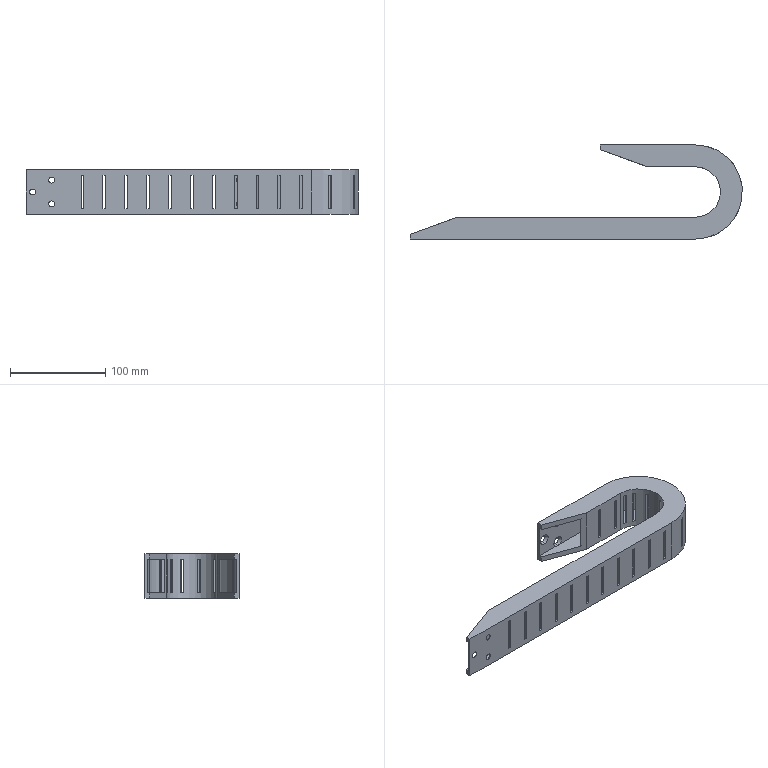Part | STEP file | TP18.35(Ruiao) | 1 solid | 146 faces | box 349.5 x 99 x 47 mm | volume 205052 mm3 | plane 118 | cylinder 16 | cone 12 | commonest cylinder face diameters 58 x7 94 x7 53 x1 99 x1